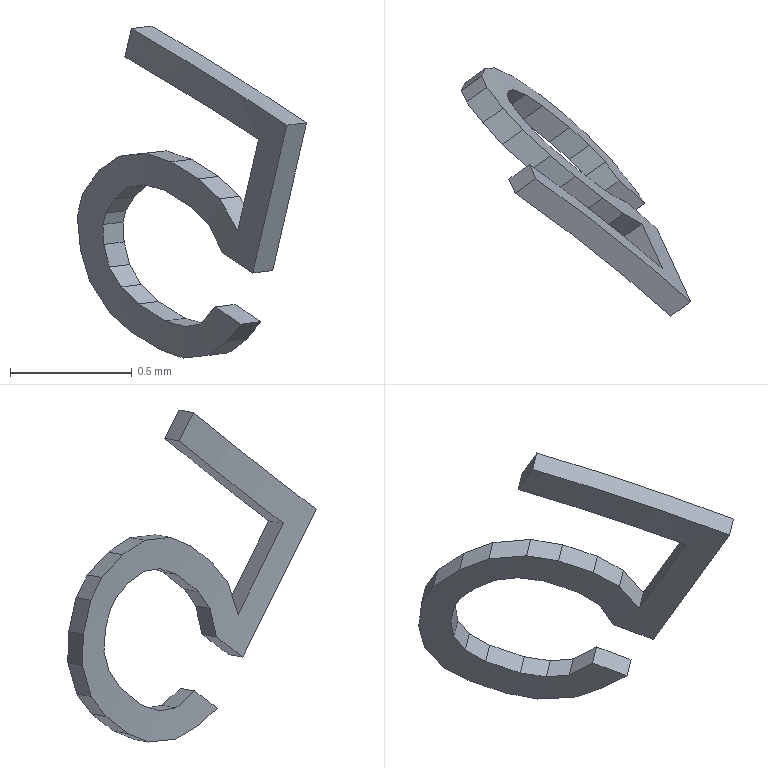Part | SolidWorks | features BaseBody 1 | 1 solid | 42 faces | box 0.9414 x 1.02 x 1.363 mm | volume 0.04689 mm3 | plane 40 | cylinder 2 | commonest cylinder face diameters 16.8 x1 17 x1